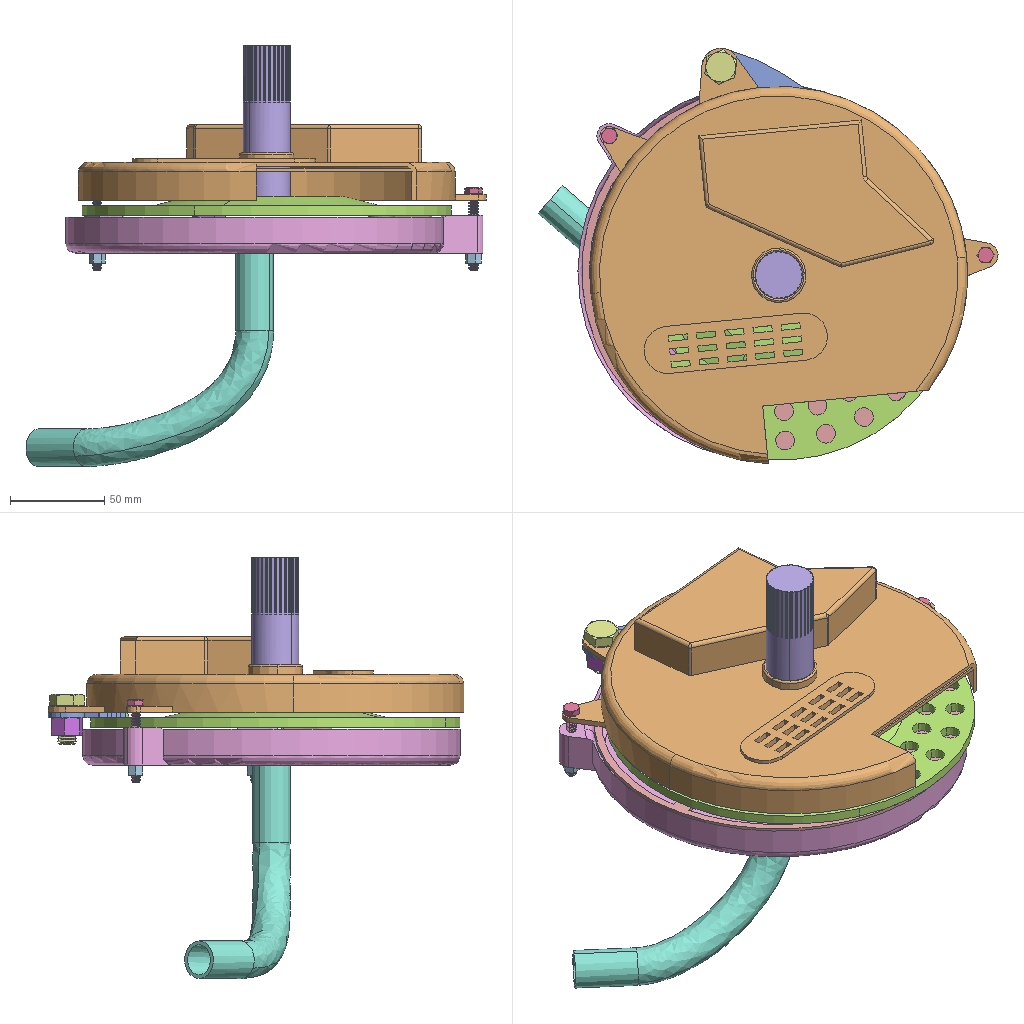Assembly | SolidWorks | 11 different items | 13 placed | box 244 x 220 x 223 mm
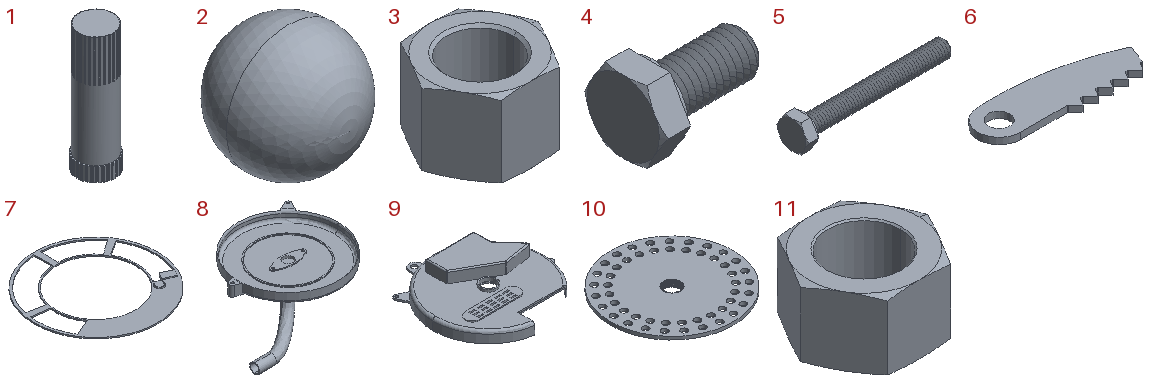Parts list (item | quantity | size | volume | features):
1 | x1 | 26.982 x 27 x 90 mm | 44504 mm3 | features CirPattern 2, ICE 2, Extrusion 1
2 | x1 | 10 x 10 x 10 mm | 523.599 mm3 | features 3DProfileFeature 1, Revolution 1
3 | x2 | 8.63 x 7.474 x 5.6 mm | 159.862 mm3 | features Cut 2, Chamfer 1, Extrusion 1
4 | x1 | 26.4 x 18.475 x 16 mm | 2601 mm3 | features RevCut 4, Chamfer 1, Extrusion 1, Fillet 1, LPattern 1, Revolution 1
5 | x2 | 43.5 x 9.238 x 8 mm | 779.159 mm3 | features RevCut 4, Chamfer 1, Extrusion 1, Fillet 1, LPattern 1, Revolution 1
6 | x1 | 70.059 x 23.839 x 3 mm | 3412 mm3 | features Extrusion 1, ICE 1
7 | x1 | 196 x 196 x 4 mm | 17953 mm3 | features ICE 4, Extrusion 1, Fillet 1
8 | x1 | 216.698 x 200 x 133.163 mm | 149560 mm3 | features ICE 6, 3DProfileFeature 2, Fillet 2, Extrusion 1, Shell 1, Sweep 1
9 | x1 | 216.698 x 221.641 x 40 mm | 144146 mm3 | features ICE 11, Fillet 3, Cut 1, Extrusion 1, Shell 1
10 | x1 | 196 x 196 x 10 mm | 165832 mm3 | features ICE 3, Blend 1, CirPattern 1, Extrusion 1
11 | x1 | 17.59 x 15.233 x 9.5 mm | 1158 mm3 | features Cut 2, Chamfer 1, Extrusion 1
Mates (type | each side: item.copy, entity, surface, feature):
Concentric | 7.1 face cylinder Boss-Extrude1 | 8.1 face cylinder Cut-Extrude3 | 2 times
Concentric | 6.1 face cylinder Cut-Extrude1 | 9.1 face cylinder Cut-Extrude9
Coincident | 6.1 face plane Boss-Extrude3 | 9.1 face plane Boss-Extrude1
Coincident | 7.1 face plane Boss-Extrude1 | 8.1 edge
Concentric | 10.1 face cylinder Cut-Extrude2 | 9.1 face cylinder Cut-Extrude7
Coincident | 6.1 face plane Boss-Extrude3 | 10.1 face plane Boss-Extrude1
Coincident | 10.1 face plane Boss-Extrude1 | 8.1 face plane Boss-Extrude1
Concentric | 8.1 face cylinder Cut-Extrude1 | 9.1 face cylinder Cut-Extrude3 | 2 times
Concentric | 9.1 face cylinder Cut-Extrude7 | 1.1 face cylinder Boss-Extrude1
Coincident | 10.1 face plane CirPattern1 | 1.1 face plane CirPattern4
Coincident | 10.1 edge | 1.1 face cylinder CirPattern4
Coincident | 10.1 face plane Loft1 | 1.1 face plane CirPattern4
Concentric | 10.1 face cylinder Cut-Extrude1 | 2.1 face sphere Revolve1
Path | 2.1 select_type:25 | assembly select_type:0
Concentric | 9.1 face cylinder Cut-Extrude3 | 5.1 face cone LPattern1
Coincident | 9.1 face plane Boss-Extrude5 | 5.1 face plane Boss-Extrude
Concentric | 9.1 face cylinder Cut-Extrude3 | 5.2 face cone LPattern1
Coincident | 9.1 face plane Boss-Extrude5 | 5.2 face plane Boss-Extrude
Concentric | 5.1 face cone LPattern1 | 3.1 face cylinder Boss-Extrude
Coincident | 8.1 face plane Boss-Extrude1 | 3.1 face plane Boss-Extrude
Concentric | 5.2 edge | 3.2 face cylinder Boss-Extrude
Coincident | 8.1 face plane Boss-Extrude1 | 3.2 face plane Boss-Extrude
Concentric | 9.1 face cylinder Cut-Extrude9 | 4.1 face cone LPattern1
Coincident | 9.1 face plane Boss-Extrude12 | 4.1 face plane Boss-Extrude
Concentric | 4.1 edge | 11.1 face cylinder Boss-Extrude
Coincident | 6.1 face plane Boss-Extrude3 | 11.1 face plane Boss-Extrude